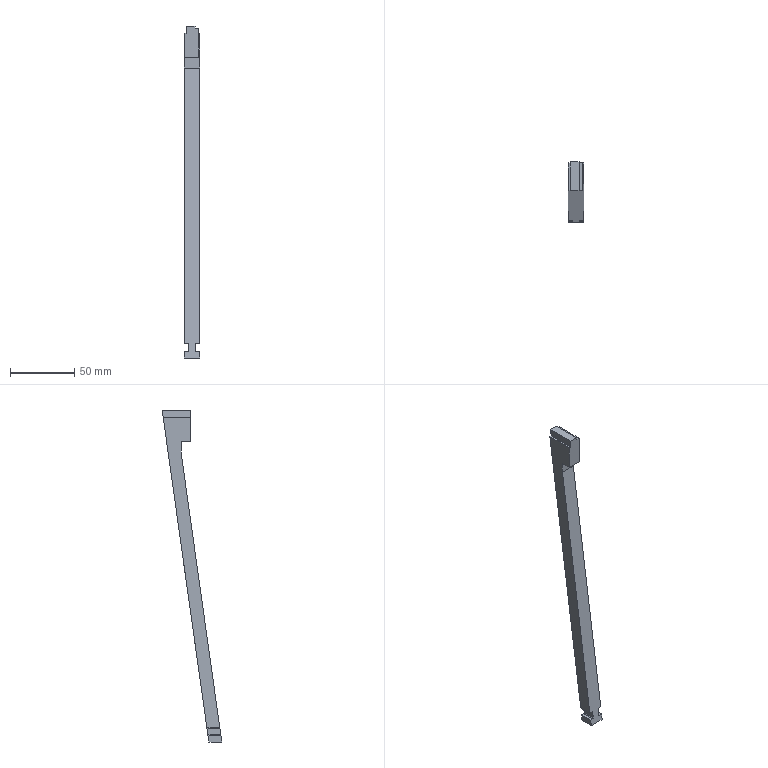Part | Creo | 1 solid | 113 faces | box 12 x 46.477 x 258.85 mm | volume 33568 mm3 | other 65 | plane 43 | cylinder 5 | commonest cylinder face diameters 1 x4 22.418 x1